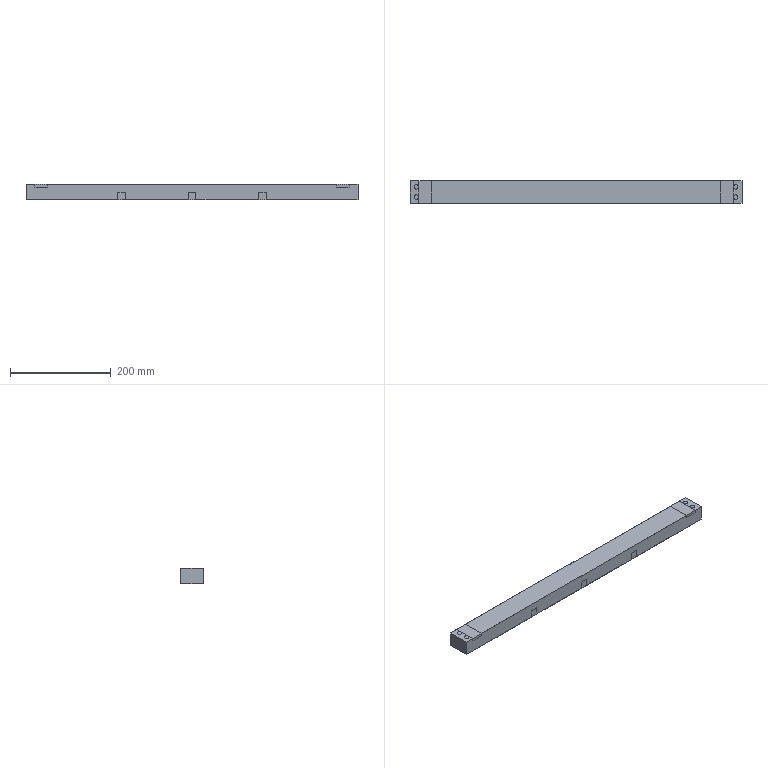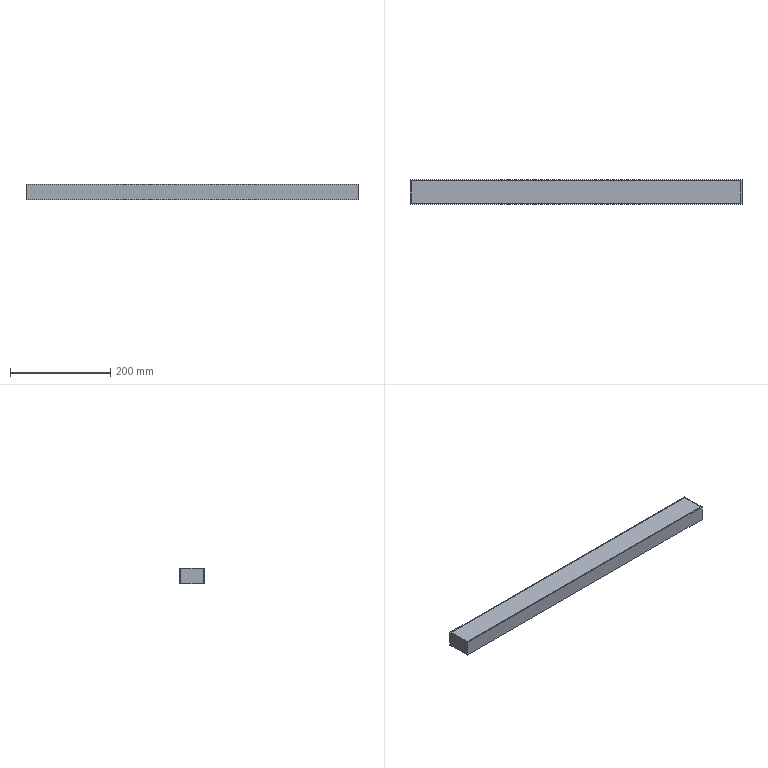CAM job | NX | 3-axis milling, drilling | part box 659.9 x 45 x 30 mm | stock box 663.9 x 49 x 31 mm
Tools:
number,name,description,diameter,corner_radius,flute_length,length,flutes
1,D63,,63.0,0.0,50.0,75.0,2
20,D12,,12.0,0.0,50.0,75.0,2
2,D6A45,,6.0,0.0,3.0,3.0,2
9,9.0ZT,,9.0,0.0,35.0,50.0,2
12,7.8ZT,,7.8,0.0,35.0,50.0,2
13,8.0JD,,8.0,0.0,30.0,30.0,4
21,D12JING,,12.0,0.0,50.0,75.0,2
10,D10,,10.0,0.0,50.0,75.0,2
5,D50,,50.0,0.0,50.0,105.0,2
Operations:
program,operation,operation_type,tool,method,geometry_group,spindle_rpm,surface_speed,feed_per_tooth,feed_cut,feed_plunge,cut_length_mm,path_length_mm,cut_time_min,machine_time_min
1,FLOOR_WALL,VolumeBased25DMillingOperation,D63,METHOD,A,6500.0,1286.0,0.0962,1250.0,1250.0,738.9,792.9,0.5911,0.5965
1,ZLEVEL_PROFILE_COPY_2,ZLevelMilling,D12,METHOD,A,8000.0,251.0,0.2188,3500.0,3500.0,4148.699,5068.442,1.185,1.277
1,FLOOR_WALL_1_2,VolumeBased25DMillingOperation,D12,METHOD,A,8000.0,251.0,0.1875,3000.0,1000.0,1740.8,2476.798,0.6283,0.7019
1,DRILLING_COPY_1,Operation,D6A45,METHOD,A,3000.0,56.0,0.0333,200.0,0.0,40.0,901.177,0.2,0.2861
1,DRILLING_COPY_COPY_1,Operation,9.0ZT,METHOD,A,1500.0,42.0,0.0667,200.0,0.0,243.6,1285.985,1.218,1.322
1,DRILLING_COPY_COPY_COPY_1,Operation,7.8ZT,METHOD,A,1500.0,42.0,0.0667,200.0,0.0,63.487,813.181,0.3174,0.3924
1,DRILLING_COPY_COPY_COPY_COPY_1,Operation,8.0JD,METHOD,A,1000.0,25.0,0.0125,50.0,0.0,56.8,799.807,1.136,1.21
1,FLOOR_WALL_1_COPY,VolumeBased25DMillingOperation,D12JING,METHOD,A,8000.0,251.0,0.075,1200.0,1000.0,380.398,1103.664,0.318,0.3903
1,CUTTERCOMP11_COPY,ZLevelMilling,D12JING,METHOD,A,8000.0,251.0,0.075,1200.0,1200.0,264.399,1273.846,0.2203,0.3213
1,CUTTERCOMP11_COPY_COPY,ZLevelMilling,D12JING,METHOD,A,8000.0,251.0,0.075,1200.0,1200.0,266.246,1146.715,0.2219,0.3099
1,ZLEVEL_PROFILE_COPY_1_COPY_COPY_COPY_COPY_2,ZLevelMilling,D6A45,METHOD,A,7000.0,131.0,0.0714,1000.0,1000.0,1622.643,4621.557,1.623,1.923
1,ZLEVEL_PROFILE_COPY_1_COPY_COPY_COPY_COPY_2_COPY,ZLevelMilling,D6A45,METHOD,A,7000.0,131.0,0.0714,1000.0,1000.0,211.165,4066.841,0.2112,0.5967
2,HOLE_MILLING,CylinderMilling,D10,METHOD,B,7000.0,219.0,0.1429,2000.0,2000.0,1108.86,2372.198,0.5544,0.6808
2,111,ZLevelMilling,D10,METHOD,B,8000.0,251.0,0.075,1200.0,1200.0,438.089,1161.897,0.3651,0.4375
2,PLANAR_MILL,PlanarMilling,D6A45,METHOD,B,8000.0,150.0,0.0781,1250.0,1250.0,1852.727,3255.985,1.482,1.623
30-45-690,FLOOR_WALL_1,VolumeBased25DMillingOperation,D63,METHOD,B,6500.0,1286.0,0.0962,1250.0,1250.0,734.9,788.9,0.5879,0.5933
CUT,ZLEVEL_PROFILE_COPY_2_1,ZLevelMilling,D50,METHOD,C,6500.0,1021.0,0.1538,2000.0,2000.0,1985.335,2107.335,0.9927,1.005